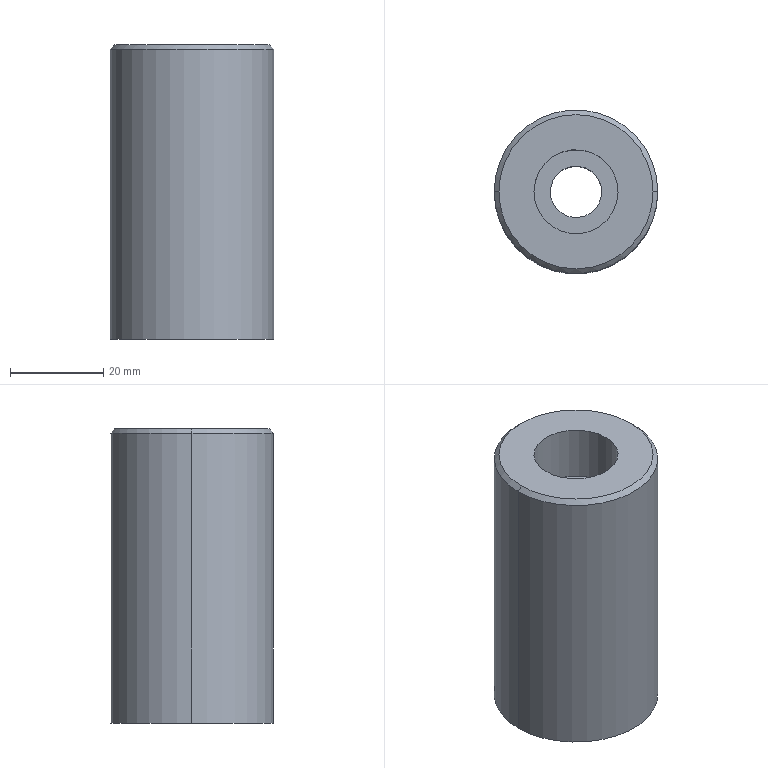Part | CATIA | 1 solid | 11 faces | box 35 x 35 x 63 mm | volume 52659 mm3 | cylinder 6 | plane 3 | cone 2 | commonest cylinder face diameters 11 x2 18 x2 35 x2
STEP:
#1=CARTESIAN_POINT('',(17.5,0.,0.));
#2=VERTEX_POINT('',#1);
#3=CARTESIAN_POINT('',(17.5,0.,62.));
#4=VERTEX_POINT('',#3);
#5=CARTESIAN_POINT('',(17.5,0.,31.5));
#6=DIRECTION('',(0.,0.,1.));
#7=VECTOR('',#6,1.);
#8=LINE('',#5,#7);
#9=EDGE_CURVE('',#2,#4,#8,.T.);
#10=ORIENTED_EDGE('',*,*,#9,.F.);
#11=CARTESIAN_POINT('',(-17.5,0.,0.));
#12=VERTEX_POINT('',#11);
#13=CARTESIAN_POINT('',(0.,0.,0.));
#14=DIRECTION('',(0.,0.,1.));
#15=AXIS2_PLACEMENT_3D('',#13,#14,$);
#16=CIRCLE('',#15,17.5);
#17=EDGE_CURVE('',#2,#12,#16,.T.);
#18=ORIENTED_EDGE('',*,*,#17,.T.);
#19=CARTESIAN_POINT('',(-17.5,0.,62.));
#20=VERTEX_POINT('',#19);
#21=CARTESIAN_POINT('',(-17.5,0.,31.5));
#22=DIRECTION('',(0.,0.,1.));
#23=VECTOR('',#22,1.);
#24=LINE('',#21,#23);
#25=EDGE_CURVE('',#12,#20,#24,.T.);
#26=ORIENTED_EDGE('',*,*,#25,.T.);
#27=CARTESIAN_POINT('',(0.,0.,62.));
#28=DIRECTION('',(0.,0.,1.));
#29=AXIS2_PLACEMENT_3D('',#27,#28,$);
#30=CIRCLE('',#29,17.5);
#31=EDGE_CURVE('',#4,#20,#30,.T.);
#32=ORIENTED_EDGE('',*,*,#31,.F.);
#33=EDGE_LOOP('',(#10,#18,#26,#32));
#34=FACE_OUTER_BOUND('',#33,.T.);
#35=CARTESIAN_POINT('',(0.,0.,31.5));
#36=DIRECTION('',(0.,0.,1.));
#37=DIRECTION('',(1.,0.,0.));
#38=AXIS2_PLACEMENT_3D('',#35,#36,#37);
#39=CYLINDRICAL_SURFACE('',#38,17.5);
#40=ADVANCED_FACE('',(#34),#39,.T.);
#41=ORIENTED_EDGE('',*,*,#25,.F.);
#42=CARTESIAN_POINT('',(0.,0.,0.));
#43=DIRECTION('',(0.,0.,1.));
#44=AXIS2_PLACEMENT_3D('',#42,#43,$);
#45=CIRCLE('',#44,17.5);
#46=EDGE_CURVE('',#12,#2,#45,.T.);
#47=ORIENTED_EDGE('',*,*,#46,.T.);
#48=ORIENTED_EDGE('',*,*,#9,.T.);
#49=CARTESIAN_POINT('',(0.,0.,62.));
#50=DIRECTION('',(0.,0.,1.));
#51=AXIS2_PLACEMENT_3D('',#49,#50,$);
#52=CIRCLE('',#51,17.5);
#53=EDGE_CURVE('',#20,#4,#52,.T.);
#54=ORIENTED_EDGE('',*,*,#53,.F.);
#55=EDGE_LOOP('',(#41,#47,#48,#54));
#56=FACE_OUTER_BOUND('',#55,.T.);
#57=ADVANCED_FACE('',(#56),#39,.T.);
#58=CARTESIAN_POINT('',(-16.5,0.00000026,63.));
#59=VERTEX_POINT('',#58);
#60=CARTESIAN_POINT('',(-17.,0.,62.5));
#61=DIRECTION('',(-0.7071,0.,-0.7071));
#62=VECTOR('',#61,1.);
#63=LINE('',#60,#62);
#64=EDGE_CURVE('',#59,#20,#63,.T.);
#65=ORIENTED_EDGE('',*,*,#64,.T.);
#66=ORIENTED_EDGE('',*,*,#53,.T.);
#67=CARTESIAN_POINT('',(16.5,0.,63.));
#68=VERTEX_POINT('',#67);
#69=CARTESIAN_POINT('',(17.,0.,62.5));
#70=DIRECTION('',(0.7071,0.,-0.7071));
#71=VECTOR('',#70,1.);
#72=LINE('',#69,#71);
#73=EDGE_CURVE('',#68,#4,#72,.T.);
#74=ORIENTED_EDGE('',*,*,#73,.F.);
#75=CARTESIAN_POINT('',(0.,0.,63.));
#76=DIRECTION('',(0.,0.,1.));
#77=AXIS2_PLACEMENT_3D('',#75,#76,$);
#78=CIRCLE('',#77,16.5);
#79=EDGE_CURVE('',#59,#68,#78,.T.);
#80=ORIENTED_EDGE('',*,*,#79,.F.);
#81=EDGE_LOOP('',(#65,#66,#74,#80));
#82=FACE_OUTER_BOUND('',#81,.T.);
#83=CARTESIAN_POINT('',(0.,0.,79.5));
#84=DIRECTION('',(0.,0.,-1.));
#85=DIRECTION('',(-0.9997,0.02581,0.));
#86=AXIS2_PLACEMENT_3D('',#83,#84,#85);
#87=CONICAL_SURFACE('',#86,0.,0.7854);
#88=ADVANCED_FACE('',(#82),#87,.T.);
#89=ORIENTED_EDGE('',*,*,#73,.T.);
#90=ORIENTED_EDGE('',*,*,#31,.T.);
#91=ORIENTED_EDGE('',*,*,#64,.F.);
#92=CARTESIAN_POINT('',(0.,0.,63.));
#93=DIRECTION('',(0.,0.,1.));
#94=AXIS2_PLACEMENT_3D('',#92,#93,$);
#95=CIRCLE('',#94,16.5);
#96=EDGE_CURVE('',#68,#59,#95,.T.);
#97=ORIENTED_EDGE('',*,*,#96,.F.);
#98=EDGE_LOOP('',(#89,#90,#91,#97));
#99=FACE_OUTER_BOUND('',#98,.T.);
#100=CARTESIAN_POINT('',(0.,0.,79.5));
#101=DIRECTION('',(0.,0.,-1.));
#102=DIRECTION('',(1.,0.,0.));
#103=AXIS2_PLACEMENT_3D('',#100,#101,#102);
#104=CONICAL_SURFACE('',#103,0.,0.7854);
#105=ADVANCED_FACE('',(#99),#104,.T.);
#106=ORIENTED_EDGE('',*,*,#79,.T.);
#107=ORIENTED_EDGE('',*,*,#96,.T.);
#108=EDGE_LOOP('',(#106,#107));
#109=FACE_OUTER_BOUND('',#108,.T.);
#110=CARTESIAN_POINT('',(7.898,-4.315,63.));
#111=VERTEX_POINT('',#110);
#112=CARTESIAN_POINT('',(-7.898,4.315,63.));
#113=VERTEX_POINT('',#112);
#114=CARTESIAN_POINT('',(0.,0.,63.));
#115=DIRECTION('',(0.,0.,1.));
#116=AXIS2_PLACEMENT_3D('',#114,#115,$);
#117=CIRCLE('',#116,9.);
#118=EDGE_CURVE('',#111,#113,#117,.T.);
#119=ORIENTED_EDGE('',*,*,#118,.F.);
#120=CARTESIAN_POINT('',(0.,0.,63.));
#121=DIRECTION('',(0.,0.,1.));
#122=AXIS2_PLACEMENT_3D('',#120,#121,$);
#123=CIRCLE('',#122,9.);
#124=EDGE_CURVE('',#113,#111,#123,.T.);
#125=ORIENTED_EDGE('',*,*,#124,.F.);
#126=EDGE_LOOP('',(#119,#125));
#127=FACE_BOUND('',#126,.T.);
#128=CARTESIAN_POINT('',(0.,0.,63.));
#129=DIRECTION('',(0.,0.,1.));
#130=DIRECTION('',(1.,0.,0.));
#131=AXIS2_PLACEMENT_3D('',#128,#129,#130);
#132=PLANE('',#131);
#133=ADVANCED_FACE('',(#109,#127),#132,.T.);
#134=ORIENTED_EDGE('',*,*,#46,.F.);
#135=ORIENTED_EDGE('',*,*,#17,.F.);
#136=EDGE_LOOP('',(#134,#135));
#137=FACE_OUTER_BOUND('',#136,.T.);
#138=CARTESIAN_POINT('',(-4.827,2.637,0.));
#139=VERTEX_POINT('',#138);
#140=CARTESIAN_POINT('',(4.827,-2.637,0.));
#141=VERTEX_POINT('',#140);
#142=CARTESIAN_POINT('',(0.,0.,0.));
#143=DIRECTION('',(0.,0.,1.));
#144=AXIS2_PLACEMENT_3D('',#142,#143,$);
#145=CIRCLE('',#144,5.5);
#146=EDGE_CURVE('',#139,#141,#145,.T.);
#147=ORIENTED_EDGE('',*,*,#146,.T.);
#148=CARTESIAN_POINT('',(0.,0.,0.));
#149=DIRECTION('',(0.,0.,1.));
#150=AXIS2_PLACEMENT_3D('',#148,#149,$);
#151=CIRCLE('',#150,5.5);
#152=EDGE_CURVE('',#141,#139,#151,.T.);
#153=ORIENTED_EDGE('',*,*,#152,.T.);
#154=EDGE_LOOP('',(#147,#153));
#155=FACE_BOUND('',#154,.T.);
#156=CARTESIAN_POINT('',(0.,0.,0.));
#157=DIRECTION('',(0.,0.,1.));
#158=DIRECTION('',(1.,0.,0.));
#159=AXIS2_PLACEMENT_3D('',#156,#157,#158);
#160=PLANE('',#159);
#161=ADVANCED_FACE('',(#137,#155),#160,.F.);
#162=CARTESIAN_POINT('',(7.898,-4.315,51.));
#163=VERTEX_POINT('',#162);
#164=CARTESIAN_POINT('',(-7.898,4.315,51.));
#165=VERTEX_POINT('',#164);
#166=CARTESIAN_POINT('',(0.,0.,51.));
#167=DIRECTION('',(0.,0.,-1.));
#168=AXIS2_PLACEMENT_3D('',#166,#167,$);
#169=CIRCLE('',#168,9.);
#170=EDGE_CURVE('',#163,#165,#169,.T.);
#171=ORIENTED_EDGE('',*,*,#170,.F.);
#172=CARTESIAN_POINT('',(0.,0.,51.));
#173=DIRECTION('',(0.,0.,-1.));
#174=AXIS2_PLACEMENT_3D('',#172,#173,$);
#175=CIRCLE('',#174,9.);
#176=EDGE_CURVE('',#165,#163,#175,.T.);
#177=ORIENTED_EDGE('',*,*,#176,.F.);
#178=EDGE_LOOP('',(#171,#177));
#179=FACE_OUTER_BOUND('',#178,.T.);
#180=CARTESIAN_POINT('',(-4.827,2.637,51.));
#181=VERTEX_POINT('',#180);
#182=CARTESIAN_POINT('',(4.827,-2.637,51.));
#183=VERTEX_POINT('',#182);
#184=CARTESIAN_POINT('',(0.,0.,51.));
#185=DIRECTION('',(0.,0.,-1.));
#186=AXIS2_PLACEMENT_3D('',#184,#185,$);
#187=CIRCLE('',#186,5.5);
#188=EDGE_CURVE('',#181,#183,#187,.T.);
#189=ORIENTED_EDGE('',*,*,#188,.T.);
#190=CARTESIAN_POINT('',(0.,0.,51.));
#191=DIRECTION('',(0.,0.,-1.));
#192=AXIS2_PLACEMENT_3D('',#190,#191,$);
#193=CIRCLE('',#192,5.5);
#194=EDGE_CURVE('',#183,#181,#193,.T.);
#195=ORIENTED_EDGE('',*,*,#194,.T.);
#196=EDGE_LOOP('',(#189,#195));
#197=FACE_BOUND('',#196,.T.);
#198=CARTESIAN_POINT('',(5.5,0.,51.));
#199=DIRECTION('',(0.,0.,-1.));
#200=DIRECTION('',(1.,0.,0.));
#201=AXIS2_PLACEMENT_3D('',#198,#199,#200);
#202=PLANE('',#201);
#203=ADVANCED_FACE('',(#179,#197),#202,.F.);
#204=ORIENTED_EDGE('',*,*,#118,.T.);
#205=CARTESIAN_POINT('',(-7.898,4.315,57.2));
#206=DIRECTION('',(0.,0.,-1.));
#207=VECTOR('',#206,1.);
#208=LINE('',#205,#207);
#209=EDGE_CURVE('',#165,#113,#208,.F.);
#210=ORIENTED_EDGE('',*,*,#209,.F.);
#211=ORIENTED_EDGE('',*,*,#176,.T.);
#212=CARTESIAN_POINT('',(7.898,-4.315,57.2));
#213=DIRECTION('',(0.,0.,-1.));
#214=VECTOR('',#213,1.);
#215=LINE('',#212,#214);
#216=EDGE_CURVE('',#163,#111,#215,.F.);
#217=ORIENTED_EDGE('',*,*,#216,.T.);
#218=EDGE_LOOP('',(#204,#210,#211,#217));
#219=FACE_OUTER_BOUND('',#218,.T.);
#220=CARTESIAN_POINT('',(0.,0.,62.9));
#221=DIRECTION('',(0.,0.,-1.));
#222=DIRECTION('',(0.8776,-0.4794,0.));
#223=AXIS2_PLACEMENT_3D('',#220,#221,#222);
#224=CYLINDRICAL_SURFACE('',#223,9.);
#225=ADVANCED_FACE('',(#219),#224,.F.);
#226=ORIENTED_EDGE('',*,*,#124,.T.);
#227=ORIENTED_EDGE('',*,*,#216,.F.);
#228=ORIENTED_EDGE('',*,*,#170,.T.);
#229=ORIENTED_EDGE('',*,*,#209,.T.);
#230=EDGE_LOOP('',(#226,#227,#228,#229));
#231=FACE_OUTER_BOUND('',#230,.T.);
#232=ADVANCED_FACE('',(#231),#224,.F.);
#233=ORIENTED_EDGE('',*,*,#146,.F.);
#234=CARTESIAN_POINT('',(-4.827,2.637,25.3));
#235=DIRECTION('',(0.,0.,-1.));
#236=VECTOR('',#235,1.);
#237=LINE('',#234,#236);
#238=EDGE_CURVE('',#139,#181,#237,.F.);
#239=ORIENTED_EDGE('',*,*,#238,.T.);
#240=ORIENTED_EDGE('',*,*,#194,.F.);
#241=CARTESIAN_POINT('',(4.827,-2.637,25.3));
#242=DIRECTION('',(0.,0.,-1.));
#243=VECTOR('',#242,1.);
#244=LINE('',#241,#243);
#245=EDGE_CURVE('',#141,#183,#244,.F.);
#246=ORIENTED_EDGE('',*,*,#245,.F.);
#247=EDGE_LOOP('',(#233,#239,#240,#246));
#248=FACE_OUTER_BOUND('',#247,.T.);
#249=CARTESIAN_POINT('',(0.,0.,62.9));
#250=DIRECTION('',(0.,0.,-1.));
#251=DIRECTION('',(0.8776,-0.4794,0.));
#252=AXIS2_PLACEMENT_3D('',#249,#250,#251);
#253=CYLINDRICAL_SURFACE('',#252,5.5);
#254=ADVANCED_FACE('',(#248),#253,.F.);
#255=ORIENTED_EDGE('',*,*,#152,.F.);
#256=ORIENTED_EDGE('',*,*,#245,.T.);
#257=ORIENTED_EDGE('',*,*,#188,.F.);
#258=ORIENTED_EDGE('',*,*,#238,.F.);
#259=EDGE_LOOP('',(#255,#256,#257,#258));
#260=FACE_OUTER_BOUND('',#259,.T.);
#261=ADVANCED_FACE('',(#260),#253,.F.);
#262=CLOSED_SHELL('',(#40,#57,#88,#105,#133,#161,#203,#225,#232,#254,#261));
#263=MANIFOLD_SOLID_BREP('',#262);
#264=(LENGTH_UNIT()NAMED_UNIT(*)SI_UNIT(.MILLI.,.METRE.));
#265=UNCERTAINTY_MEASURE_WITH_UNIT(LENGTH_MEASURE(0.005),#264,'','');
#266=(NAMED_UNIT(*)PLANE_ANGLE_UNIT()SI_UNIT($,.RADIAN.));
#267=(NAMED_UNIT(*)SI_UNIT($,.STERADIAN.)SOLID_ANGLE_UNIT());
#268=(GEOMETRIC_REPRESENTATION_CONTEXT(3)GLOBAL_UNCERTAINTY_ASSIGNED_CONTEXT((#265))GLOBAL_UNIT_ASSIGNED_CONTEXT((#264,#266,#267))REPRESENTATION_CONTEXT('',''));
#269=ADVANCED_BREP_SHAPE_REPRESENTATION('',(#263),#268);